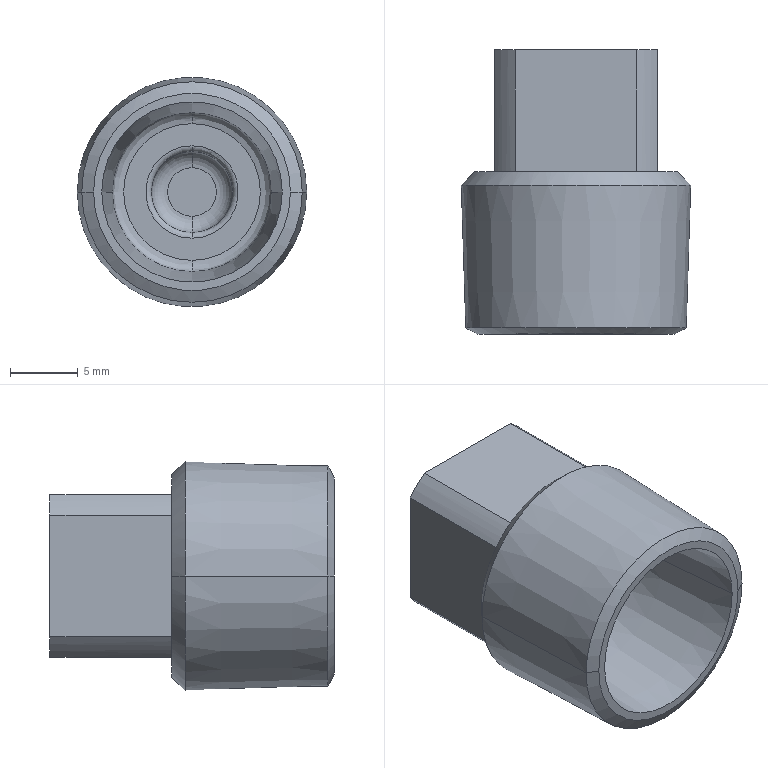Part | STEP file | SUCPP10A | 1 solid | 29 faces | box 16.949 x 21 x 16.949 mm | volume 2402 mm3 | plane 9 | cone 8 | torus 6 | cylinder 6 | commonest cylinder face diameters 15 x4 6 x2